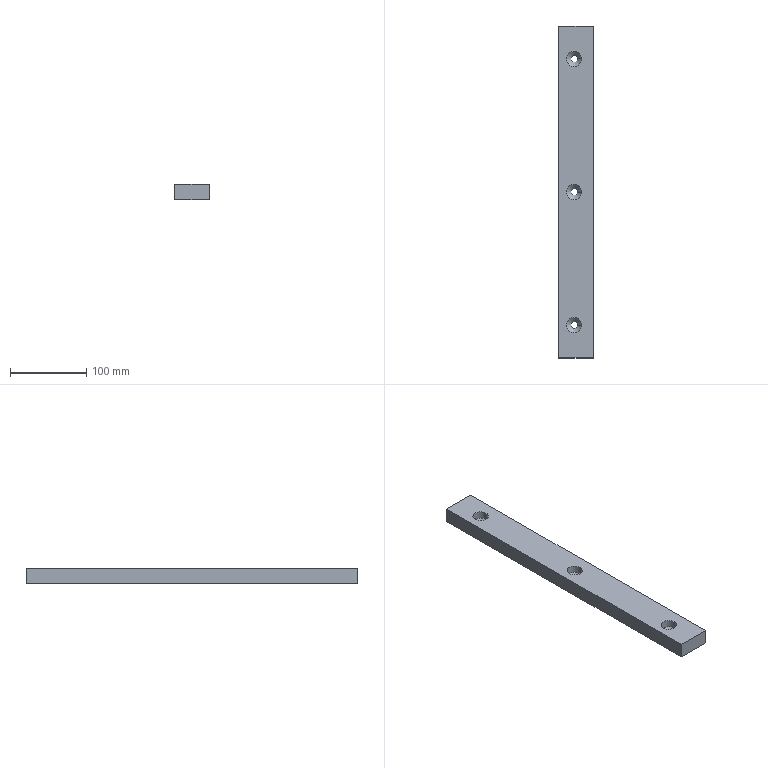Part | STEP file | 1 solid | 24 faces | box 45 x 436.5 x 20 mm | volume 379711 mm3 | cylinder 12 | plane 6 | cone 6 | commonest cylinder face diameters 9 x6 20 x6